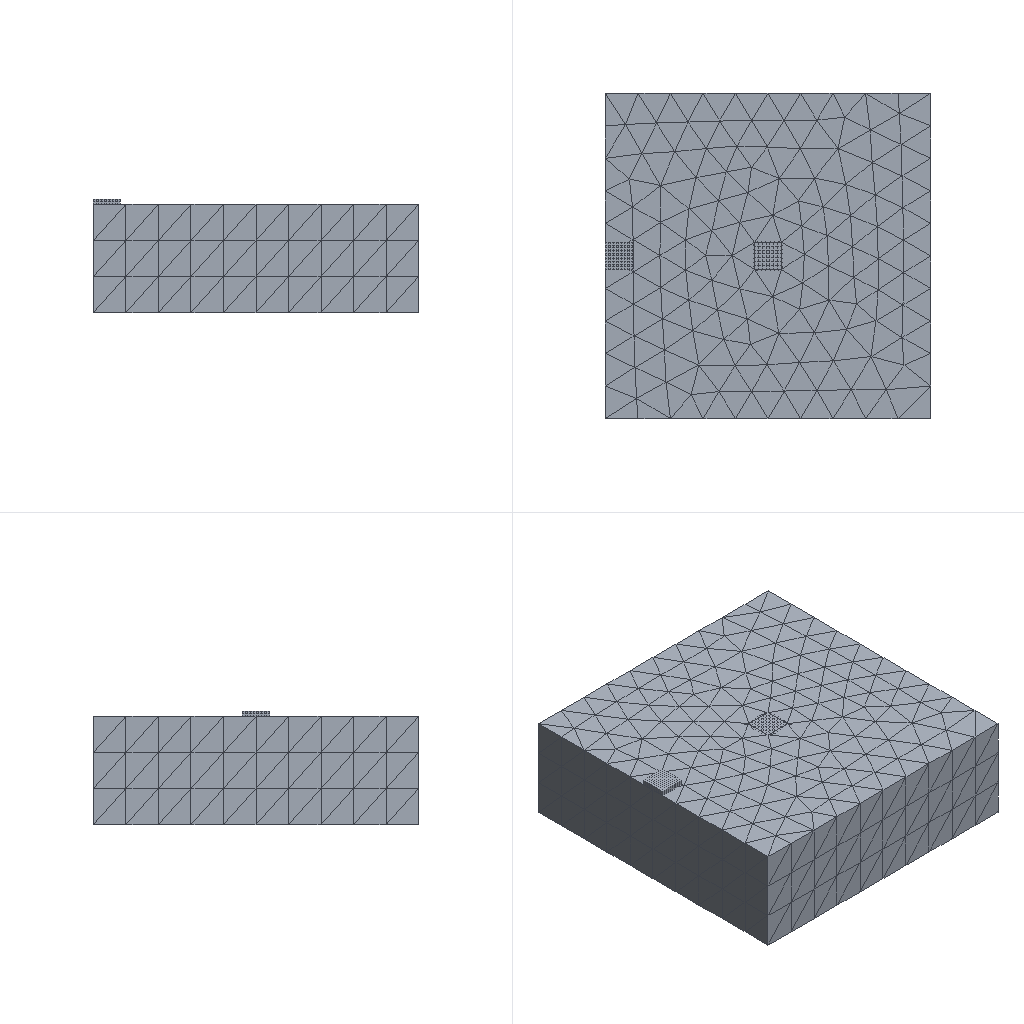Simulation study | abaqus
Set-up summary:
category,name,step,type,value,unit,region
solver,abaqus,,Abaqus/CAE 2024
units,SI m-kg-s (Pa),,inferred,E=1.2e+10 density=7850
analysis,Step-1,,dynamic implicit,nlgeom=True; time_period=1
mesh,nodes,,,4847
mesh,elements,,,2970
element_type,C3D10,,,2574
element_type,C3D8R,,,396
material,con,,E,1.2e+10
material,con,,nu,0.35
material,con,,density,7850
material,pla,,E,3e+09
material,pla,,nu,0.38
material,pla,,density,1000
section,pla,,solid section,,,_PickedSet2
section,con,,solid section,,,_PickedSet2
section,con,,solid section,,,_PickedSet2
load,Load-1,Step-1,pressure,3.2e+06,,_PickedSurf25
bc,BC-2,initial,encastre,[dofs=ENCASTRE],,_PickedSet27
bc,BC-3,initial,fixed,[dofs=x],,_PickedSet28
bc,BC-4,initial,fixed,[dofs=y],,_PickedSet29
bc,BC-1,Step-1,displacement,2.75 [dofs=x],,_PickedSet26
bc,BC-1,Step-1,fixed,[dofs=y],,_PickedSet26
contact,Int-1,initial,general contact,interaction=IntProp-1; friction=0.2; behavior=hard
Abaqus input file, long lists of numbers shortened:
*Heading
** Job name: deck Model name: Model-1
** Generated by: Abaqus/CAE 2024
*Preprint, echo=NO, model=NO, history=NO, contact=NO
**
** PARTS
**
*Part, name=Part-4
*Node
      1, -0.345,  0.1, 0.05
      2,   -0.3093,  0.1, 0.05
** (318 more lines like these left out)
*Element, type=C3D8R
  1,  65,  66,  74,  73,   1,   2,  10,   9
  2,  66,  67,  75,  74,   2,   3,  11,  10
** (194 more lines like these left out)
*Nset, nset=_PickedSet2, internal, generate
   1,  320,    1
*Elset, elset=_PickedSet2, internal, generate
   1,  196,    1
** Section: Section-2
*Solid Section, elset=_PickedSet2, material=pla
,
*End Part
**
*Part, name=Part-5
*Node
      1,         1.75,        -1.25,  0.95
      2,         1.25,        -1.25,  0.95
** (4162 more lines like these left out)
*Element, type=C3D10
   1,  350,  351,  115,  352,  625,  624,  623,  627,  626,  628
   2,  350,  124,  353,  352,  631,  630,  629,  627,  632,  633
** (2572 more lines like these left out)
*Nset, nset=_PickedSet2, internal, generate
    1,  4164,     1
*Elset, elset=_PickedSet2, internal, generate
    1,  2574,     1
** Section: con
*Solid Section, elset=_PickedSet2, material=con
,
*End Part
**
*Part, name=Part-7
*Node
      1, -0.155, -0.06, 0.05
      2, -0.155, -0.035, 0.05
** (361 more lines like these left out)
*Element, type=C3D8R
  1,  34,  35,  46,  45,   1,   2,  13,  12
  2,  35,  36,  47,  46,   2,   3,  14,  13
** (198 more lines like these left out)
*Nset, nset=_PickedSet2, internal, generate
   1,  363,    1
*Elset, elset=_PickedSet2, internal, generate
   1,  200,    1
** Section: con
*Solid Section, elset=_PickedSet2, material=con
,
*End Part
**
**
** ASSEMBLY
**
*Assembly, name=Assembly
**
*Instance, name=Part-4-1, part=Part-4
        1.72,       -1.725,         0.95
*End Instance
**
*Instance, name=Part-5-1, part=Part-5
*End Instance
**
*Instance, name=Part-7-1, part=Part-7
       0.155,       -1.565,           1.
*End Instance
**
*Nset, nset=_PickedSet26, internal, instance=Part-7-1
   1,   2,   3,   4,   5,   6,   7,   8,   9,  10,  11,  12,  13,  14,  15,  16
  17,  18,  19,  20,  21,  22,  23,  24,  25,  26,  27,  28,  29,  30,  31,  32
** (6 more lines like these left out)
*Elset, elset=_PickedSet26, internal, instance=Part-7-1
   1,   2,   3,   4,   5,   6,   7,   8,   9,  10,  11,  12,  13,  14,  15,  16
  17,  18,  19,  20,  21,  30,  31,  40,  41,  50,  51,  60,  61,  70,  71,  80
** (3 more lines like these left out)
*Nset, nset=_PickedSet27, internal, instance=Part-5-1
    7,    8,   14,   15,   28,   29,   30,   31,   32,   33,   34,   35,   36,   50,   51,   52
   53,   54,   55,   56,   57,   58,   59,   60,   61,   62,   63,   64,   65,   66,   67,   68
** (26 more lines like these left out)
*Elset, elset=_PickedSet27, internal, instance=Part-5-1
   13,   19,   74,   92,  179,  205,  207,  253,  254,  317,  326,  370,  408,  458,  510,  546
  613,  624,  628,  653,  692,  718,  738,  763,  810,  813,  828,  830,  845,  852,  853,  886
** (11 more lines like these left out)
*Nset, nset=_PickedSet28, internal, instance=Part-5-1
    5,    6,    7,    8,   13,   14,   15,   16,   17,   18,   19,   20,   21,   22,   23,   24
   25,   26,   27,   28,   29,   30,   31,   32,   33,   34,   35,   36,   37,   38,   48,   49
** (17 more lines like these left out)
*Elset, elset=_PickedSet28, internal, instance=Part-5-1
   77,   98,  111,  140,  389,  426,  460,  462,  595,  667,  682,  693,  695,  697,  700,  712
  722,  775,  797,  825,  870,  885,  931,  973, 1034, 1117, 1134, 1157, 1168, 1173, 1189, 1277
** (6 more lines like these left out)
*Nset, nset=_PickedSet29, internal, instance=Part-5-1
    5,    6,    7,    8,   13,   14,   15,   16,   26,   27,   37,   38,   39,   40,   41,   42
   43,   44,   45,   46,   47,   48,   49,   50,   51,   52,   53,   54,   55,   56,   57,   58
** (17 more lines like these left out)
*Elset, elset=_PickedSet29, internal, instance=Part-5-1
   28,  134,  631,  638,  664,  696,  728,  733,  744,  773,  783,  799,  818,  896,  919,  923
  966,  998, 1046, 1069, 1086, 1176, 1214, 1216, 1255, 1279, 1312, 1360, 1364, 1466, 1537, 1545
** (6 more lines like these left out)
*Elset, elset=__PickedSurf25_S3, internal, instance=Part-7-1
   1,   2,   3,   4,   5,   6,   7,   8,   9,  10,  21,  22,  23,  24,  25,  26
  27,  28,  29,  30,  41,  42,  43,  44,  45,  46,  47,  48,  49,  50,  61,  62
** (5 more lines like these left out)
*Surface, type=ELEMENT, name=_PickedSurf25, internal
__PickedSurf25_S3, S3
*End Assembly
**
** MATERIALS
**
*Material, name=con
*Density
7850.,
*Elastic
 1.2e+10, 0.35
*Material, name=pla
*Density
1000.,
*Elastic
 3e+09, 0.38
**
** INTERACTION PROPERTIES
**
*Surface Interaction, name=IntProp-1
1.,
*Friction, slip tolerance=0.005
 0.2,
*Surface Behavior, pressure-overclosure=HARD
**
** BOUNDARY CONDITIONS
**
** Name: BC-2 Type: Symmetry/Antisymmetry/Encastre
*Boundary
_PickedSet27, ENCASTRE
** Name: BC-3 Type: Displacement/Rotation
*Boundary
_PickedSet28, 1, 1
** Name: BC-4 Type: Displacement/Rotation
*Boundary
_PickedSet29, 2, 2
**
** INTERACTIONS
**
** Interaction: Int-1
*Contact
*Contact Inclusions, ALL EXTERIOR
*Contact Property Assignment
 ,  , IntProp-1
** ----------------------------------------------------------------
**
** STEP: Step-1
**
*Step, name=Step-1, nlgeom=YES, inc=10000
*Dynamic
0.01,1.,1e-05
**
** BOUNDARY CONDITIONS
**
** Name: BC-1 Type: Displacement/Rotation
*Boundary
_PickedSet26, 1, 1, 2.75
_PickedSet26, 2, 2
**
** LOADS
**
** Name: Load-1   Type: Pressure
*Dsload
_PickedSurf25, P, 3.2e+06
**
** OUTPUT REQUESTS
**
*Restart, write, frequency=0
**
** FIELD OUTPUT: F-Output-1
**
*Output, field, variable=PRESELECT, frequency=1
**
** HISTORY OUTPUT: H-Output-1
**
*Output, history, variable=PRESELECT
*End Step
Results summary:
result,odb.job_status,,,JOB_STATUS_COMPLETED_SUCCESSFULLY,"consistent, unstated (Abaqus has no unit system)"
result,steps[0].procedure,Step-1,,*DYNAMIC,"consistent, unstated (Abaqus has no unit system)"
result,steps[0].time_period,Step-1,,1,"consistent, unstated (Abaqus has no unit system)"
result,steps[0].n_frames,Step-1,,25,"consistent, unstated (Abaqus has no unit system)"
result,steps[0].last_frame.id,Step-1,,24,"consistent, unstated (Abaqus has no unit system)"
result,steps[0].last_frame.value,Step-1,,1,"consistent, unstated (Abaqus has no unit system)"
result,steps[0].last_frame.description,Step-1,,Increment     24: Step Time =    1.000,"consistent, unstated (Abaqus has no unit system)"
result,steps[0].completed,Step-1,,True,"consistent, unstated (Abaqus has no unit system)"
result,steps[0].max_U_magnitude,Step-1,,2.75,"consistent, unstated (Abaqus has no unit system)"
result,steps[0].max_S_mises,Step-1,,3.29279e+06,"consistent, unstated (Abaqus has no unit system)"
result,steps[0].RF_sum[1],Step-1,,118.846,"consistent, unstated (Abaqus has no unit system)"
result,steps[0].RF_sum[2],Step-1,,0.05075,"consistent, unstated (Abaqus has no unit system)"
result,steps[0].RF_sum[3],Step-1,,200007,"consistent, unstated (Abaqus has no unit system)"